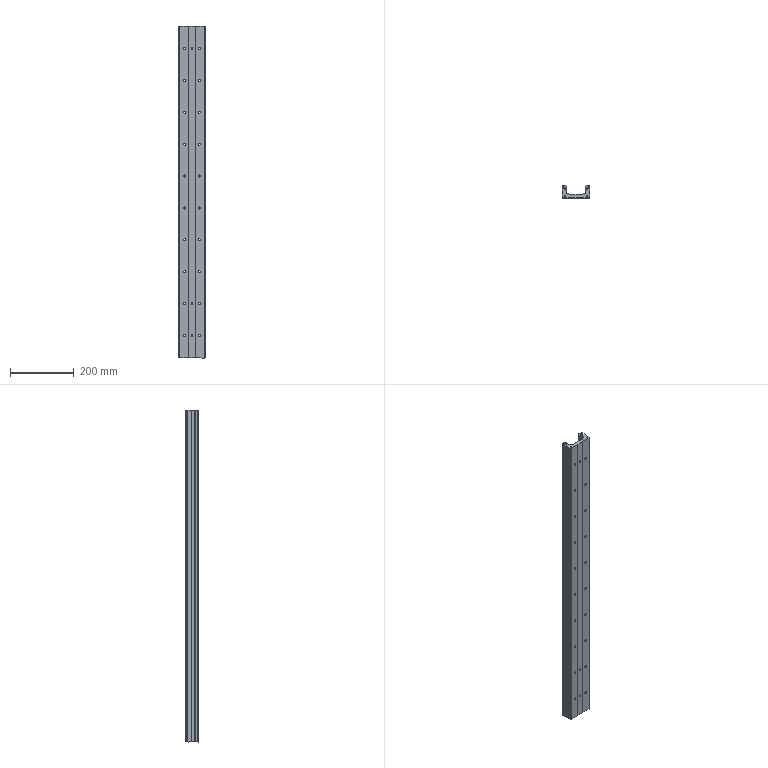Part | SolidWorks | features BaseBody 1 | 1 solid | 225 faces | box 86 x 38.5 x 1040 mm | volume 1661800 mm3 | cylinder 110 | plane 95 | cone 20 | commonest cylinder face diameters 6.6 x40 11 x40 3.3 x16 6 x9 4 x3 3 x2